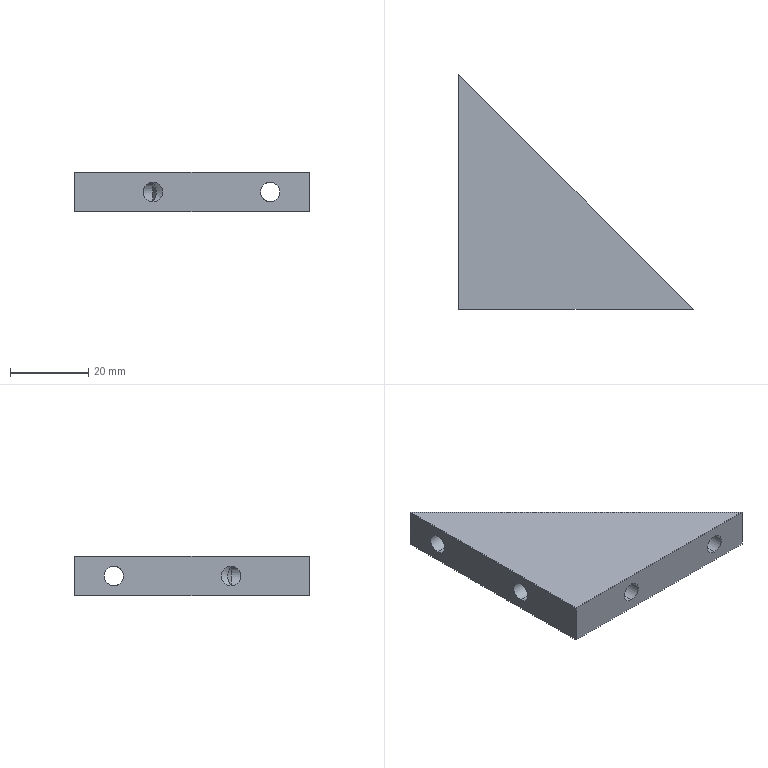Part | SolidWorks | features HoleWzd 2, Extrusion 1 | 1 solid | 15 faces | box 60 x 60 x 10 mm | volume 16836 mm3 | cylinder 8 | plane 5 | cone 2 | commonest cylinder face diameters 5 x8
STEP:
#1=CARTESIAN_POINT('',(-20.,20.,2.5));
#2=VERTEX_POINT('',#1);
#3=CARTESIAN_POINT('',(-20.,20.,7.5));
#4=VERTEX_POINT('',#3);
#5=CARTESIAN_POINT('',(-20.,20.,2.5));
#6=CARTESIAN_POINT('',(-15.,15.,2.5));
#7=CARTESIAN_POINT('',(-15.,15.,7.5));
#8=CARTESIAN_POINT('',(-20.,20.,7.5));
#9=(BOUNDED_CURVE()B_SPLINE_CURVE(3,(#5,#6,#7,#8),.UNSPECIFIED.,.F.,.F.)B_SPLINE_CURVE_WITH_KNOTS((4,4),(1.571,4.712),.UNSPECIFIED.)CURVE()GEOMETRIC_REPRESENTATION_ITEM()RATIONAL_B_SPLINE_CURVE((1.,0.3333,0.3333,1.))REPRESENTATION_ITEM(''));
#10=EDGE_CURVE('',#2,#4,#9,.T.);
#11=ORIENTED_EDGE('',*,*,#10,.F.);
#12=CARTESIAN_POINT('',(-30.,20.,2.5));
#13=VERTEX_POINT('',#12);
#14=CARTESIAN_POINT('',(-30.,20.,2.5));
#15=DIRECTION('',(-1.,0.,0.));
#16=VECTOR('',#15,1000.);
#17=LINE('',#14,#16);
#18=EDGE_CURVE('',#2,#13,#17,.T.);
#19=ORIENTED_EDGE('',*,*,#18,.T.);
#20=CARTESIAN_POINT('',(-30.,20.,7.5));
#21=VERTEX_POINT('',#20);
#22=CARTESIAN_POINT('',(-30.,20.,5.));
#23=DIRECTION('',(-1.,0.,0.));
#24=DIRECTION('',(0.,0.,1.));
#25=AXIS2_PLACEMENT_3D('',#22,#23,#24);
#26=CIRCLE('',#25,2.5);
#27=EDGE_CURVE('',#13,#21,#26,.T.);
#28=ORIENTED_EDGE('',*,*,#27,.T.);
#29=CARTESIAN_POINT('',(-30.,20.,7.5));
#30=DIRECTION('',(-1.,0.,0.));
#31=VECTOR('',#30,1000.);
#32=LINE('',#29,#31);
#33=EDGE_CURVE('',#4,#21,#32,.T.);
#34=ORIENTED_EDGE('',*,*,#33,.F.);
#35=EDGE_LOOP('',(#11,#19,#28,#34));
#36=FACE_OUTER_BOUND('',#35,.T.);
#37=CARTESIAN_POINT('',(-30.,20.,5.));
#38=DIRECTION('',(-1.,0.,0.));
#39=DIRECTION('',(0.,0.,1.));
#40=AXIS2_PLACEMENT_3D('',#37,#38,#39);
#41=CYLINDRICAL_SURFACE('',#40,2.5);
#42=ADVANCED_FACE('',(#36),#41,.F.);
#43=CARTESIAN_POINT('',(-10.,-10.,2.5));
#44=VERTEX_POINT('',#43);
#45=CARTESIAN_POINT('',(-10.,-10.,7.5));
#46=VERTEX_POINT('',#45);
#47=CARTESIAN_POINT('',(-10.,-10.,2.5));
#48=CARTESIAN_POINT('',(-15.,-15.,2.5));
#49=CARTESIAN_POINT('',(-15.,-15.,7.5));
#50=CARTESIAN_POINT('',(-10.,-10.,7.5));
#51=(BOUNDED_CURVE()B_SPLINE_CURVE(3,(#47,#48,#49,#50),.UNSPECIFIED.,.F.,.F.)B_SPLINE_CURVE_WITH_KNOTS((4,4),(4.712,7.854),.UNSPECIFIED.)CURVE()GEOMETRIC_REPRESENTATION_ITEM()RATIONAL_B_SPLINE_CURVE((1.,0.3333,0.3333,1.))REPRESENTATION_ITEM(''));
#52=EDGE_CURVE('',#44,#46,#51,.T.);
#53=ORIENTED_EDGE('',*,*,#52,.F.);
#54=CARTESIAN_POINT('',(-30.,-10.,2.5));
#55=VERTEX_POINT('',#54);
#56=CARTESIAN_POINT('',(-30.,-10.,2.5));
#57=DIRECTION('',(-1.,0.,0.));
#58=VECTOR('',#57,1000.);
#59=LINE('',#56,#58);
#60=EDGE_CURVE('',#44,#55,#59,.T.);
#61=ORIENTED_EDGE('',*,*,#60,.T.);
#62=CARTESIAN_POINT('',(-30.,-10.,7.5));
#63=VERTEX_POINT('',#62);
#64=CARTESIAN_POINT('',(-30.,-10.,5.));
#65=DIRECTION('',(-1.,0.,0.));
#66=DIRECTION('',(0.,0.,1.));
#67=AXIS2_PLACEMENT_3D('',#64,#65,#66);
#68=CIRCLE('',#67,2.5);
#69=EDGE_CURVE('',#55,#63,#68,.T.);
#70=ORIENTED_EDGE('',*,*,#69,.T.);
#71=CARTESIAN_POINT('',(-30.,-10.,7.5));
#72=DIRECTION('',(-1.,0.,0.));
#73=VECTOR('',#72,1000.);
#74=LINE('',#71,#73);
#75=EDGE_CURVE('',#46,#63,#74,.T.);
#76=ORIENTED_EDGE('',*,*,#75,.F.);
#77=EDGE_LOOP('',(#53,#61,#70,#76));
#78=FACE_OUTER_BOUND('',#77,.T.);
#79=CARTESIAN_POINT('',(-30.,-10.,5.));
#80=DIRECTION('',(-1.,0.,0.));
#81=DIRECTION('',(0.,0.,1.));
#82=AXIS2_PLACEMENT_3D('',#79,#80,#81);
#83=CYLINDRICAL_SURFACE('',#82,2.5);
#84=ADVANCED_FACE('',(#78),#83,.F.);
#85=ORIENTED_EDGE('',*,*,#52,.T.);
#86=CARTESIAN_POINT('',(-10.,-30.,7.5));
#87=VERTEX_POINT('',#86);
#88=CARTESIAN_POINT('',(-10.,-30.,7.5));
#89=DIRECTION('',(0.,-1.,0.));
#90=VECTOR('',#89,1000.);
#91=LINE('',#88,#90);
#92=EDGE_CURVE('',#46,#87,#91,.T.);
#93=ORIENTED_EDGE('',*,*,#92,.T.);
#94=CARTESIAN_POINT('',(-10.,-30.,2.5));
#95=VERTEX_POINT('',#94);
#96=CARTESIAN_POINT('',(-10.,-30.,5.));
#97=DIRECTION('',(0.,-1.,0.));
#98=DIRECTION('',(0.,0.,-1.));
#99=AXIS2_PLACEMENT_3D('',#96,#97,#98);
#100=CIRCLE('',#99,2.5);
#101=EDGE_CURVE('',#87,#95,#100,.T.);
#102=ORIENTED_EDGE('',*,*,#101,.T.);
#103=CARTESIAN_POINT('',(-10.,-30.,2.5));
#104=DIRECTION('',(0.,-1.,0.));
#105=VECTOR('',#104,1000.);
#106=LINE('',#103,#105);
#107=EDGE_CURVE('',#44,#95,#106,.T.);
#108=ORIENTED_EDGE('',*,*,#107,.F.);
#109=EDGE_LOOP('',(#85,#93,#102,#108));
#110=FACE_OUTER_BOUND('',#109,.T.);
#111=CARTESIAN_POINT('',(-10.,-30.,5.));
#112=DIRECTION('',(0.,-1.,0.));
#113=DIRECTION('',(0.,0.,-1.));
#114=AXIS2_PLACEMENT_3D('',#111,#112,#113);
#115=CYLINDRICAL_SURFACE('',#114,2.5);
#116=ADVANCED_FACE('',(#110),#115,.F.);
#117=CARTESIAN_POINT('',(20.,-20.,7.5));
#118=VERTEX_POINT('',#117);
#119=CARTESIAN_POINT('',(20.,-20.,2.5));
#120=VERTEX_POINT('',#119);
#121=CARTESIAN_POINT('',(20.,-20.,7.5));
#122=CARTESIAN_POINT('',(15.,-15.,7.5));
#123=CARTESIAN_POINT('',(15.,-15.,2.5));
#124=CARTESIAN_POINT('',(20.,-20.,2.5));
#125=(BOUNDED_CURVE()B_SPLINE_CURVE(3,(#121,#122,#123,#124),.UNSPECIFIED.,.F.,.F.)B_SPLINE_CURVE_WITH_KNOTS((4,4),(1.571,4.712),.UNSPECIFIED.)CURVE()GEOMETRIC_REPRESENTATION_ITEM()RATIONAL_B_SPLINE_CURVE((1.,0.3333,0.3333,1.))REPRESENTATION_ITEM(''));
#126=EDGE_CURVE('',#118,#120,#125,.T.);
#127=ORIENTED_EDGE('',*,*,#126,.F.);
#128=CARTESIAN_POINT('',(20.,-30.,7.5));
#129=VERTEX_POINT('',#128);
#130=CARTESIAN_POINT('',(20.,-30.,7.5));
#131=DIRECTION('',(0.,-1.,0.));
#132=VECTOR('',#131,1000.);
#133=LINE('',#130,#132);
#134=EDGE_CURVE('',#118,#129,#133,.T.);
#135=ORIENTED_EDGE('',*,*,#134,.T.);
#136=CARTESIAN_POINT('',(20.,-30.,2.5));
#137=VERTEX_POINT('',#136);
#138=CARTESIAN_POINT('',(20.,-30.,5.));
#139=DIRECTION('',(0.,-1.,0.));
#140=DIRECTION('',(0.,0.,-1.));
#141=AXIS2_PLACEMENT_3D('',#138,#139,#140);
#142=CIRCLE('',#141,2.5);
#143=EDGE_CURVE('',#129,#137,#142,.T.);
#144=ORIENTED_EDGE('',*,*,#143,.T.);
#145=CARTESIAN_POINT('',(20.,-30.,2.5));
#146=DIRECTION('',(0.,-1.,0.));
#147=VECTOR('',#146,1000.);
#148=LINE('',#145,#147);
#149=EDGE_CURVE('',#120,#137,#148,.T.);
#150=ORIENTED_EDGE('',*,*,#149,.F.);
#151=EDGE_LOOP('',(#127,#135,#144,#150));
#152=FACE_OUTER_BOUND('',#151,.T.);
#153=CARTESIAN_POINT('',(20.,-30.,5.));
#154=DIRECTION('',(0.,-1.,0.));
#155=DIRECTION('',(0.,0.,-1.));
#156=AXIS2_PLACEMENT_3D('',#153,#154,#155);
#157=CYLINDRICAL_SURFACE('',#156,2.5);
#158=ADVANCED_FACE('',(#152),#157,.F.);
#159=CARTESIAN_POINT('',(-20.,20.,7.5));
#160=CARTESIAN_POINT('',(-25.,25.,7.5));
#161=CARTESIAN_POINT('',(-25.,25.,2.5));
#162=CARTESIAN_POINT('',(-20.,20.,2.5));
#163=(BOUNDED_CURVE()B_SPLINE_CURVE(3,(#159,#160,#161,#162),.UNSPECIFIED.,.F.,.F.)B_SPLINE_CURVE_WITH_KNOTS((4,4),(4.712,7.854),.UNSPECIFIED.)CURVE()GEOMETRIC_REPRESENTATION_ITEM()RATIONAL_B_SPLINE_CURVE((1.,0.3333,0.3333,1.))REPRESENTATION_ITEM(''));
#164=EDGE_CURVE('',#4,#2,#163,.T.);
#165=ORIENTED_EDGE('',*,*,#164,.T.);
#166=ORIENTED_EDGE('',*,*,#10,.T.);
#167=EDGE_LOOP('',(#165,#166));
#168=FACE_BOUND('',#167,.T.);
#169=CARTESIAN_POINT('',(20.,-20.,2.5));
#170=CARTESIAN_POINT('',(25.,-25.,2.5));
#171=CARTESIAN_POINT('',(25.,-25.,7.5));
#172=CARTESIAN_POINT('',(20.,-20.,7.5));
#173=(BOUNDED_CURVE()B_SPLINE_CURVE(3,(#169,#170,#171,#172),.UNSPECIFIED.,.F.,.F.)B_SPLINE_CURVE_WITH_KNOTS((4,4),(4.712,7.854),.UNSPECIFIED.)CURVE()GEOMETRIC_REPRESENTATION_ITEM()RATIONAL_B_SPLINE_CURVE((1.,0.3333,0.3333,1.))REPRESENTATION_ITEM(''));
#174=EDGE_CURVE('',#120,#118,#173,.T.);
#175=ORIENTED_EDGE('',*,*,#174,.T.);
#176=ORIENTED_EDGE('',*,*,#126,.T.);
#177=EDGE_LOOP('',(#175,#176));
#178=FACE_BOUND('',#177,.T.);
#179=CARTESIAN_POINT('',(30.,-30.,0.));
#180=VERTEX_POINT('',#179);
#181=CARTESIAN_POINT('',(-30.,30.,0.));
#182=VERTEX_POINT('',#181);
#183=CARTESIAN_POINT('',(-30.,30.,0.));
#184=DIRECTION('',(-0.7071,0.7071,0.));
#185=VECTOR('',#184,1000.);
#186=LINE('',#183,#185);
#187=EDGE_CURVE('',#180,#182,#186,.T.);
#188=ORIENTED_EDGE('',*,*,#187,.T.);
#189=CARTESIAN_POINT('',(-30.,30.,10.));
#190=VERTEX_POINT('',#189);
#191=CARTESIAN_POINT('',(-30.,30.,10.));
#192=DIRECTION('',(0.,0.,-1.));
#193=VECTOR('',#192,1000.);
#194=LINE('',#191,#193);
#195=EDGE_CURVE('',#190,#182,#194,.T.);
#196=ORIENTED_EDGE('',*,*,#195,.F.);
#197=CARTESIAN_POINT('',(30.,-30.,10.));
#198=VERTEX_POINT('',#197);
#199=CARTESIAN_POINT('',(-30.,30.,10.));
#200=DIRECTION('',(-0.7071,0.7071,0.));
#201=VECTOR('',#200,1000.);
#202=LINE('',#199,#201);
#203=EDGE_CURVE('',#198,#190,#202,.T.);
#204=ORIENTED_EDGE('',*,*,#203,.F.);
#205=CARTESIAN_POINT('',(30.,-30.,10.));
#206=DIRECTION('',(0.,0.,-1.));
#207=VECTOR('',#206,1000.);
#208=LINE('',#205,#207);
#209=EDGE_CURVE('',#198,#180,#208,.T.);
#210=ORIENTED_EDGE('',*,*,#209,.T.);
#211=EDGE_LOOP('',(#188,#196,#204,#210));
#212=FACE_OUTER_BOUND('',#211,.T.);
#213=CARTESIAN_POINT('',(-30.,30.,10.));
#214=DIRECTION('',(-0.7071,-0.7071,0.));
#215=DIRECTION('',(0.7071,-0.7071,0.));
#216=AXIS2_PLACEMENT_3D('',#213,#214,#215);
#217=PLANE('',#216);
#218=ADVANCED_FACE('',(#168,#178,#212),#217,.F.);
#219=CARTESIAN_POINT('',(-30.,20.,5.));
#220=DIRECTION('',(-1.,0.,0.));
#221=DIRECTION('',(0.,0.,1.));
#222=AXIS2_PLACEMENT_3D('',#219,#220,#221);
#223=CIRCLE('',#222,2.5);
#224=EDGE_CURVE('',#21,#13,#223,.T.);
#225=ORIENTED_EDGE('',*,*,#224,.F.);
#226=ORIENTED_EDGE('',*,*,#27,.F.);
#227=EDGE_LOOP('',(#225,#226));
#228=FACE_BOUND('',#227,.T.);
#229=CARTESIAN_POINT('',(-30.,-10.,5.));
#230=DIRECTION('',(-1.,0.,0.));
#231=DIRECTION('',(0.,0.,1.));
#232=AXIS2_PLACEMENT_3D('',#229,#230,#231);
#233=CIRCLE('',#232,2.5);
#234=EDGE_CURVE('',#63,#55,#233,.T.);
#235=ORIENTED_EDGE('',*,*,#234,.F.);
#236=ORIENTED_EDGE('',*,*,#69,.F.);
#237=EDGE_LOOP('',(#235,#236));
#238=FACE_BOUND('',#237,.T.);
#239=CARTESIAN_POINT('',(-30.,-30.,0.));
#240=VERTEX_POINT('',#239);
#241=CARTESIAN_POINT('',(-30.,30.,0.));
#242=DIRECTION('',(0.,-1.,0.));
#243=VECTOR('',#242,1000.);
#244=LINE('',#241,#243);
#245=EDGE_CURVE('',#182,#240,#244,.T.);
#246=ORIENTED_EDGE('',*,*,#245,.T.);
#247=CARTESIAN_POINT('',(-30.,-30.,10.));
#248=VERTEX_POINT('',#247);
#249=CARTESIAN_POINT('',(-30.,-30.,10.));
#250=DIRECTION('',(0.,0.,-1.));
#251=VECTOR('',#250,1000.);
#252=LINE('',#249,#251);
#253=EDGE_CURVE('',#248,#240,#252,.T.);
#254=ORIENTED_EDGE('',*,*,#253,.F.);
#255=CARTESIAN_POINT('',(-30.,30.,10.));
#256=DIRECTION('',(0.,-1.,0.));
#257=VECTOR('',#256,1000.);
#258=LINE('',#255,#257);
#259=EDGE_CURVE('',#190,#248,#258,.T.);
#260=ORIENTED_EDGE('',*,*,#259,.F.);
#261=ORIENTED_EDGE('',*,*,#195,.T.);
#262=EDGE_LOOP('',(#246,#254,#260,#261));
#263=FACE_OUTER_BOUND('',#262,.T.);
#264=CARTESIAN_POINT('',(-30.,30.,10.));
#265=DIRECTION('',(1.,0.,0.));
#266=DIRECTION('',(0.,1.,0.));
#267=AXIS2_PLACEMENT_3D('',#264,#265,#266);
#268=PLANE('',#267);
#269=ADVANCED_FACE('',(#228,#238,#263),#268,.F.);
#270=CARTESIAN_POINT('',(-10.,-30.,5.));
#271=DIRECTION('',(0.,-1.,0.));
#272=DIRECTION('',(0.,0.,-1.));
#273=AXIS2_PLACEMENT_3D('',#270,#271,#272);
#274=CIRCLE('',#273,2.5);
#275=EDGE_CURVE('',#95,#87,#274,.T.);
#276=ORIENTED_EDGE('',*,*,#275,.F.);
#277=ORIENTED_EDGE('',*,*,#101,.F.);
#278=EDGE_LOOP('',(#276,#277));
#279=FACE_BOUND('',#278,.T.);
#280=CARTESIAN_POINT('',(20.,-30.,5.));
#281=DIRECTION('',(0.,-1.,0.));
#282=DIRECTION('',(0.,0.,-1.));
#283=AXIS2_PLACEMENT_3D('',#280,#281,#282);
#284=CIRCLE('',#283,2.5);
#285=EDGE_CURVE('',#137,#129,#284,.T.);
#286=ORIENTED_EDGE('',*,*,#285,.F.);
#287=ORIENTED_EDGE('',*,*,#143,.F.);
#288=EDGE_LOOP('',(#286,#287));
#289=FACE_BOUND('',#288,.T.);
#290=CARTESIAN_POINT('',(-30.,-30.,0.));
#291=DIRECTION('',(1.,0.,0.));
#292=VECTOR('',#291,1000.);
#293=LINE('',#290,#292);
#294=EDGE_CURVE('',#240,#180,#293,.T.);
#295=ORIENTED_EDGE('',*,*,#294,.T.);
#296=ORIENTED_EDGE('',*,*,#209,.F.);
#297=CARTESIAN_POINT('',(-30.,-30.,10.));
#298=DIRECTION('',(1.,0.,0.));
#299=VECTOR('',#298,1000.);
#300=LINE('',#297,#299);
#301=EDGE_CURVE('',#248,#198,#300,.T.);
#302=ORIENTED_EDGE('',*,*,#301,.F.);
#303=ORIENTED_EDGE('',*,*,#253,.T.);
#304=EDGE_LOOP('',(#295,#296,#302,#303));
#305=FACE_OUTER_BOUND('',#304,.T.);
#306=CARTESIAN_POINT('',(-30.,-30.,10.));
#307=DIRECTION('',(0.,1.,0.));
#308=DIRECTION('',(0.,0.,1.));
#309=AXIS2_PLACEMENT_3D('',#306,#307,#308);
#310=PLANE('',#309);
#311=ADVANCED_FACE('',(#279,#289,#305),#310,.F.);
#312=ORIENTED_EDGE('',*,*,#203,.T.);
#313=ORIENTED_EDGE('',*,*,#259,.T.);
#314=ORIENTED_EDGE('',*,*,#301,.T.);
#315=EDGE_LOOP('',(#312,#313,#314));
#316=FACE_OUTER_BOUND('',#315,.T.);
#317=CARTESIAN_POINT('',(0.,0.,10.));
#318=DIRECTION('',(0.,0.,1.));
#319=DIRECTION('',(1.,0.,0.));
#320=AXIS2_PLACEMENT_3D('',#317,#318,#319);
#321=PLANE('',#320);
#322=ADVANCED_FACE('',(#316),#321,.T.);
#323=ORIENTED_EDGE('',*,*,#187,.F.);
#324=ORIENTED_EDGE('',*,*,#294,.F.);
#325=ORIENTED_EDGE('',*,*,#245,.F.);
#326=EDGE_LOOP('',(#323,#324,#325));
#327=FACE_OUTER_BOUND('',#326,.T.);
#328=CARTESIAN_POINT('',(0.,0.,0.));
#329=DIRECTION('',(0.,0.,1.));
#330=DIRECTION('',(1.,0.,0.));
#331=AXIS2_PLACEMENT_3D('',#328,#329,#330);
#332=PLANE('',#331);
#333=ADVANCED_FACE('',(#327),#332,.F.);
#334=ORIENTED_EDGE('',*,*,#134,.F.);
#335=ORIENTED_EDGE('',*,*,#174,.F.);
#336=ORIENTED_EDGE('',*,*,#149,.T.);
#337=ORIENTED_EDGE('',*,*,#285,.T.);
#338=EDGE_LOOP('',(#334,#335,#336,#337));
#339=FACE_OUTER_BOUND('',#338,.T.);
#340=CARTESIAN_POINT('',(20.,-30.,5.));
#341=DIRECTION('',(0.,-1.,0.));
#342=DIRECTION('',(0.,0.,-1.));
#343=AXIS2_PLACEMENT_3D('',#340,#341,#342);
#344=CYLINDRICAL_SURFACE('',#343,2.5);
#345=ADVANCED_FACE('',(#339),#344,.F.);
#346=CARTESIAN_POINT('',(-10.,-10.,5.));
#347=DIRECTION('',(0.,-1.,0.));
#348=DIRECTION('',(0.,0.,-1.));
#349=AXIS2_PLACEMENT_3D('',#346,#347,#348);
#350=CIRCLE('',#349,2.5);
#351=EDGE_CURVE('',#44,#46,#350,.T.);
#352=ORIENTED_EDGE('',*,*,#351,.T.);
#353=CARTESIAN_POINT('',(-10.,-10.,7.5));
#354=CARTESIAN_POINT('',(-9.89,-9.89,7.316));
#355=CARTESIAN_POINT('',(-9.782,-9.782,7.13));
#356=CARTESIAN_POINT('',(-9.575,-9.575,6.747));
#357=CARTESIAN_POINT('',(-9.476,-9.476,6.551));
#358=CARTESIAN_POINT('',(-9.296,-9.296,6.14));
#359=CARTESIAN_POINT('',(-9.216,-9.216,5.927));
#360=CARTESIAN_POINT('',(-9.127,-9.127,5.588));
#361=CARTESIAN_POINT('',(-9.103,-9.103,5.471));
#362=CARTESIAN_POINT('',(-9.07,-9.07,5.235));
#363=CARTESIAN_POINT('',(-9.061,-9.061,5.116));
#364=CARTESIAN_POINT('',(-9.062,-9.062,4.752));
#365=CARTESIAN_POINT('',(-9.099,-9.099,4.515));
#366=CARTESIAN_POINT('',(-9.22,-9.22,4.061));
#367=CARTESIAN_POINT('',(-9.3,-9.3,3.851));
#368=CARTESIAN_POINT('',(-9.567,-9.567,3.243));
#369=CARTESIAN_POINT('',(-9.78,-9.78,2.866));
#370=CARTESIAN_POINT('',(-10.,-10.,2.5));
#371=B_SPLINE_CURVE_WITH_KNOTS('',3,(#353,#354,#355,#356,#357,#358,#359,#360,#361,#362,#363,#364,#365,#366,#367,#368,#369,#370),.UNSPECIFIED.,.F.,.F.,(4,2,2,2,2,2,2,2,4),(0.000000262,0.0007226,0.001445,0.002167,0.002528,0.00289,0.003612,0.004334,0.005779),.UNSPECIFIED.);
#372=EDGE_CURVE('',#46,#44,#371,.T.);
#373=ORIENTED_EDGE('',*,*,#372,.T.);
#374=EDGE_LOOP('',(#352,#373));
#375=FACE_OUTER_BOUND('',#374,.T.);
#376=CARTESIAN_POINT('',(-10.,-10.,5.));
#377=DIRECTION('',(0.,-1.,0.));
#378=DIRECTION('',(0.,0.,-1.));
#379=AXIS2_PLACEMENT_3D('',#376,#377,#378);
#380=CONICAL_SURFACE('',#379,2.5,1.03);
#381=ADVANCED_FACE('',(#375),#380,.F.);
#382=ORIENTED_EDGE('',*,*,#92,.F.);
#383=ORIENTED_EDGE('',*,*,#351,.F.);
#384=ORIENTED_EDGE('',*,*,#107,.T.);
#385=ORIENTED_EDGE('',*,*,#275,.T.);
#386=EDGE_LOOP('',(#382,#383,#384,#385));
#387=FACE_OUTER_BOUND('',#386,.T.);
#388=CARTESIAN_POINT('',(-10.,-30.,5.));
#389=DIRECTION('',(0.,-1.,0.));
#390=DIRECTION('',(0.,0.,-1.));
#391=AXIS2_PLACEMENT_3D('',#388,#389,#390);
#392=CYLINDRICAL_SURFACE('',#391,2.5);
#393=ADVANCED_FACE('',(#387),#392,.F.);
#394=ORIENTED_EDGE('',*,*,#60,.F.);
#395=CARTESIAN_POINT('',(-10.,-10.,5.));
#396=DIRECTION('',(-1.,0.,0.));
#397=DIRECTION('',(0.,0.,1.));
#398=AXIS2_PLACEMENT_3D('',#395,#396,#397);
#399=CIRCLE('',#398,2.5);
#400=EDGE_CURVE('',#46,#44,#399,.T.);
#401=ORIENTED_EDGE('',*,*,#400,.F.);
#402=ORIENTED_EDGE('',*,*,#75,.T.);
#403=ORIENTED_EDGE('',*,*,#234,.T.);
#404=EDGE_LOOP('',(#394,#401,#402,#403));
#405=FACE_OUTER_BOUND('',#404,.T.);
#406=CARTESIAN_POINT('',(-30.,-10.,5.));
#407=DIRECTION('',(-1.,0.,0.));
#408=DIRECTION('',(0.,0.,1.));
#409=AXIS2_PLACEMENT_3D('',#406,#407,#408);
#410=CYLINDRICAL_SURFACE('',#409,2.5);
#411=ADVANCED_FACE('',(#405),#410,.F.);
#412=ORIENTED_EDGE('',*,*,#400,.T.);
#413=ORIENTED_EDGE('',*,*,#372,.F.);
#414=EDGE_LOOP('',(#412,#413));
#415=FACE_OUTER_BOUND('',#414,.T.);
#416=CARTESIAN_POINT('',(-10.,-10.,5.));
#417=DIRECTION('',(-1.,0.,0.));
#418=DIRECTION('',(0.,0.,1.));
#419=AXIS2_PLACEMENT_3D('',#416,#417,#418);
#420=CONICAL_SURFACE('',#419,2.5,1.03);
#421=ADVANCED_FACE('',(#415),#420,.F.);
#422=ORIENTED_EDGE('',*,*,#18,.F.);
#423=ORIENTED_EDGE('',*,*,#164,.F.);
#424=ORIENTED_EDGE('',*,*,#33,.T.);
#425=ORIENTED_EDGE('',*,*,#224,.T.);
#426=EDGE_LOOP('',(#422,#423,#424,#425));
#427=FACE_OUTER_BOUND('',#426,.T.);
#428=CARTESIAN_POINT('',(-30.,20.,5.));
#429=DIRECTION('',(-1.,0.,0.));
#430=DIRECTION('',(0.,0.,1.));
#431=AXIS2_PLACEMENT_3D('',#428,#429,#430);
#432=CYLINDRICAL_SURFACE('',#431,2.5);
#433=ADVANCED_FACE('',(#427),#432,.F.);
#434=CLOSED_SHELL('',(#42,#84,#116,#158,#218,#269,#311,#322,#333,#345,#381,#393,#411,#421,#433));
#435=MANIFOLD_SOLID_BREP('',#434);
#436=CARTESIAN_POINT('',(0.,0.,0.));
#437=DIRECTION('',(0.,0.,1.));
#438=DIRECTION('',(1.,0.,0.));
#439=AXIS2_PLACEMENT_3D('',#436,#437,#438);
#440=(LENGTH_UNIT()NAMED_UNIT(*)SI_UNIT(.MILLI.,.METRE.));
#441=UNCERTAINTY_MEASURE_WITH_UNIT(LENGTH_MEASURE(0.00001),#440,'','');
#442=(NAMED_UNIT(*)PLANE_ANGLE_UNIT()SI_UNIT($,.RADIAN.));
#443=(NAMED_UNIT(*)SI_UNIT($,.STERADIAN.)SOLID_ANGLE_UNIT());
#444=(GEOMETRIC_REPRESENTATION_CONTEXT(3)GLOBAL_UNCERTAINTY_ASSIGNED_CONTEXT((#441))GLOBAL_UNIT_ASSIGNED_CONTEXT((#440,#442,#443))REPRESENTATION_CONTEXT('',''));
#445=ADVANCED_BREP_SHAPE_REPRESENTATION('',(#435,#439),#444);